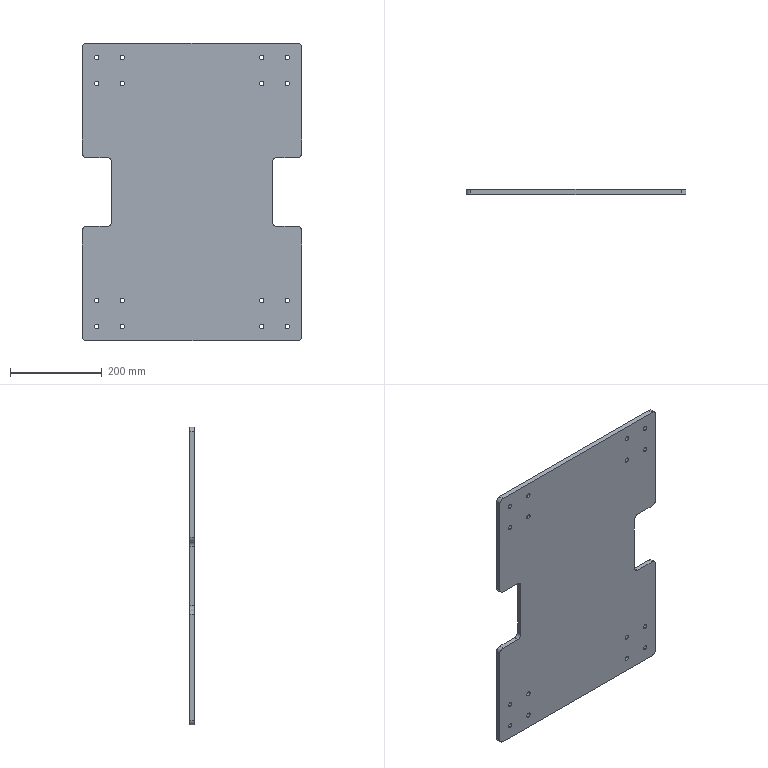Part | SolidWorks | features Fillet 2, ICE 2, Extrusion 1 | 1 solid | 58 faces | box 480 x 10 x 650 mm | volume 2911575 mm3 | cylinder 44 | plane 14 | commonest cylinder face diameters 10 x32 20 x12